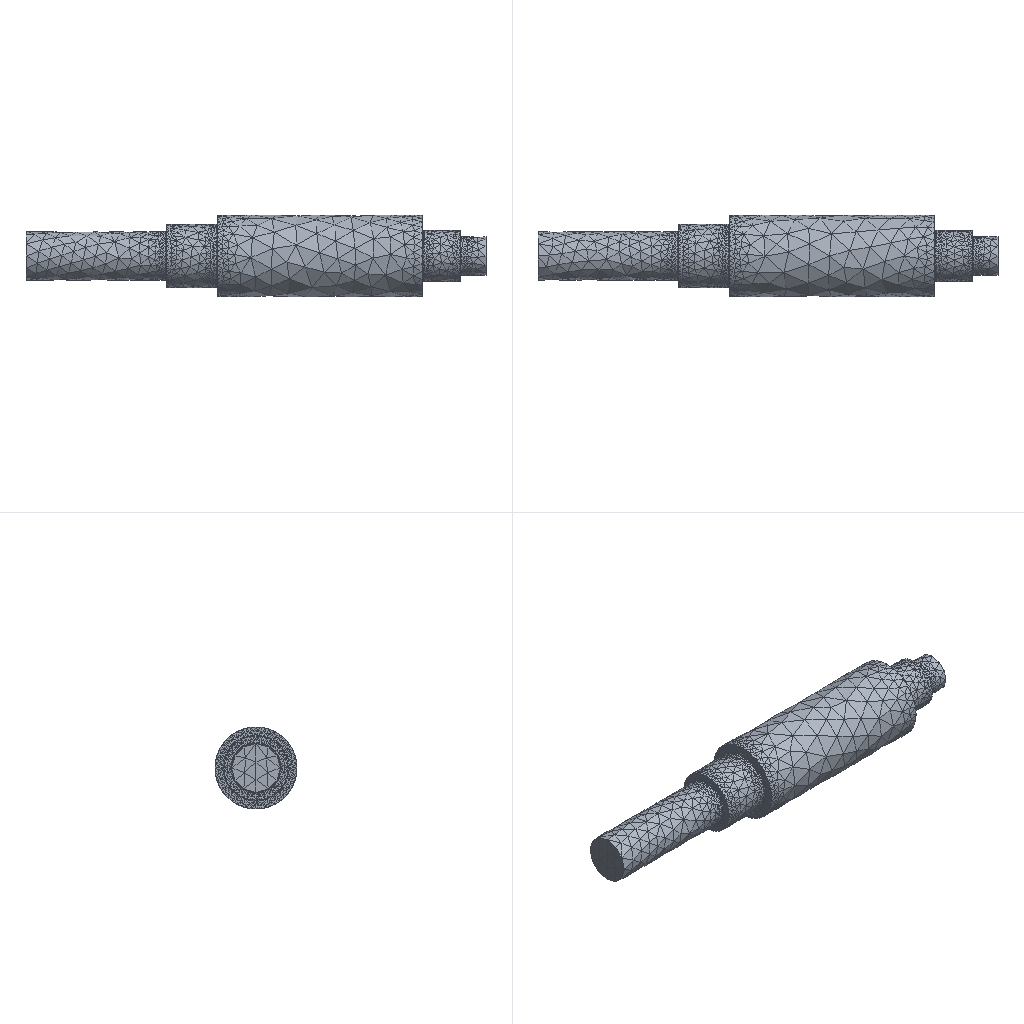Simulation study | ansys workbench
Set-up summary:
category,name,step,type,value,unit,region
solver,ansys_workbench
units,mm-N-s-tonne (MPa),,stated,"/units,MPA"
analysis,LS1,,modal,method=lanb; n_modes=20
load_step,LS1,LS1,modal
mesh,nodes,,,91403
mesh,elements,,,61675
element_type,SOLID187,,,61675
material,Structural Steel,,E,200000,tonne s^-2 mm^-1
material,Structural Steel,,nu,0.3
material,Structural Steel,,density,7.85e-09,tonne mm^-3
material,Structural Steel,,conductivity,60.5,tonne mm s^-3 C^-1
material,Structural Steel,,specific_heat,4.34e+08,mm^2 s^-2 C^-1
material,Structural Steel,,cte,1.2e-05,C^-1
material,Structural Steel,,permeability,10000
material,Structural Steel,,resistivity,0.00017,ohm mm
bc,Frictionless Supports X,model,fixed,[dofs=UX],,_FRICSUX
bc,Frictionless Supports Z,model,fixed,[dofs=UZ],,_FRICSUZ
named_set,_FRICSUX,,node,2114
named_set,_FRICSUZ,,node,2114
Ansys APDL input file, long lists of numbers shortened:
/batch
/config,noeldb,1     ! force off writing results to database
*get,_wallstrt,active,,time,wall
! ANSYS input file written by Workbench version 2025 R2
! File used for geometry attach:
/title,______________--__ (A5)
! ****** Begin Custom Load Command Snippet ******
/COM, ACT Extensions:
/COM,     LSDYNA, 2025.2
/COM,/COM,     ANSYSMotion, 2025.2
/COM,
! ****** End   Custom Load Command Snippet ******
*DIM,_wb_ProjectScratch_dir,string,248
_wb_ProjectScratch_dir(1) = ''
/com,--- Data in consistent NMM units. See Solving Units in the help system for more information.
/units,MPA
/nopr
/wb,file,start              !  signify a WB generated input file
/prep7
! Turn off shape checking because checks already performed inside WB mesher.
! See help system for more information.
SHPP,OFF,,NOWARN
/nolist
etcon,set             ! allow ANSYS to choose best KEYOP's for 180x elements, resets any applicable keyopt to MAPDL defaults
/com,*********** Send User Defined Coordinate System(s) ***********
csys,0
/com,*********** Nodes for the whole assembly ***********
nblock,3,,100543
(1i9,3e20.9e3)
        1     0.000000000E+00    -1.163414459E-15    -9.500000000E+00
! (91402 more lines like these left out)
-1
/wb,elem,start            !  set before creation of elements
/com,*********** Elements for Body 1 'Part 1' ***********
et,1,187
MAT,1 $ TYPE,1 $ REAL,1 $ SECNUM,1 $ ESYS,0
eblock,11,COMPACT,,61675
(11i9)
        1     7993    12675     8526     9142    67015    70402    67012    67013    74710    70396
! (61674 more lines like these left out)
-1
secnum,1    ! reset the section ID to default
/wb,elem,end               !  done creating elements
toffst,273.15,      ! Temperature offset from absolute zero
/com,*********** Set Reference Temperature ***********
tref,22.
/wb,mat,start              !  starting to send materials
/com,*********** Send Materials ***********
Temperature = 'TEMP' ! Temperature
MP,DENS,1,7.85e-09,	! tonne mm^-3
MP,ALPX,1,1.2e-05,	! C^-1
MP,C,1,434000000,	! mm^2 s^-2 C^-1
MP,KXX,1,60.5,	! tonne mm s^-3 C^-1
MP,RSVX,1,0.00017,	! ohm mm
MP,EX,1,200000,	! tonne s^-2 mm^-1
MP,NUXY,1,0.3,
MP,MURX,1,10000,
/wb,mat,end                !  done sending materials
!************************* Model Summary ********************
!Part 1,	结构钢,	matid,	1
!************************* End Model Summary ********************
! get the diagonal of the bounding box. Needed later for other things
*get,_xmin,node,,mnloc,x
*get,_ymin,node,,mnloc,y
*get,_zmin,node,,mnloc,z
*get,_xmax,node,,mxloc,x
*get,_ymax,node,,mxloc,y
*get,_zmax,node,,mxloc,z
_ASMDIAG=(_xmax-_xmin)*(_xmax-_xmin)+(_ymax-_ymin)*(_ymax-_ymin)+(_zmax-_zmin)*(_zmax-_zmin)
_ASMDIAG=SQRT(_ASMDIAG)
/wb,contact,start          !  starting to send contact
/wb,contact,end            !  done creating contacts
/golist
/wb,load,start             !  starting to send loads
/com,********* Frictionless Supports X *********
CMBLOCK,_FRICSUX,NODE,     2114
(8i10)
       262      -473      1125     -1234      1753     -1981      2597     -3039
! (264 more lines like these left out)
cmsel,s,_FRICSUX
d,all,ux,0
nsel,all
/com,********* Frictionless Supports Z *********
CMBLOCK,_FRICSUZ,NODE,     2114
(8i10)
       262      -473      1125     -1234      1753     -1981      2597     -3039
! (264 more lines like these left out)
cmsel,s,_FRICSUZ
d,all,uz,0
nsel,all
/com,*********** Node Rotations ***********
nmod,262,,,,-180.,0.,90.
nmod,263,,,,-180.,7.66,90.
nmod,264,,,,-180.,15.319,90.
nmod,265,,,,-180.,22.979,90.
! (3650 more lines like these left out)
/gst,on,on
fini
*get,_numnode,node,0,count
*get,_numelem,elem,0,count
*get, _MAXELEMNUM, elem, 0, NUM, MAX
*get, _MAXNODENUM, node, 0, NUM, MAX
*get, _MAXELEMTYPE, etyp, 0, NUM, MAX
*get, _MAXREALCONST, rcon, 0, NUM, MAX
/go
/wb,load,end               !  done creating loads
/com,--- Number of total nodes = %_numnode%
/com,--- Number of contact elements = 0
/com,--- Number of spring elements = 0
/com,--- Number of bearing elements = 0
/com,--- Number of solid elements = 61675
/com,--- Number of condensed parts = 0
/com,--- Number of total elements = %_numelem%
*get,_wallbsol,active,,time,wall
/solu
antype,2                   ! modal analysis
_thickRatio=  1     ! Ratio of thick parts in the model
thexpand,off     ! ignore thermal strains
modopt,lanb,20
outres,erase
outres,all,none
outres,nsol,all
outres,strs,all,
outres,epel,all,
outres,eppl,all,
mxpand,,,,yes,,no             ! expand requested element results, but not write them to file.mode
dmpopt,esav,no
dmpopt,emat,no
dmpopt,full,no
! *********** WB SOLVE COMMAND ***********
! check interactive state
*get,ANSINTER_,active,,int
*if,ANSINTER_,ne,0,then
/eof
*endif
solve
/com *************** Write FE CONNECTORS *********
CEWRITE,file,ce,,INTE
*get,_nmodalsolproc,active,0,numcpu
fini
/nopr
*get,_numnode,node,0,count
*get,_numelem,elem,0,count
*get, _MAXELEMNUM, elem, 0, NUM, MAX
*get, _MAXNODENUM, node, 0, NUM, MAX,,,INTERNAL
*get, _MAXELEMTYPE, etyp, 0, NUM, MAX
*get, _MAXREALCONST, rcon, 0, NUM, MAX
*get,_NSOLTHREADS,active,0,ntfs
*get,_NSOLPROCESSES,active,0,npfs
/gopr
*get,_wallasol,active,,time,wall
/post1
/nopr
*dim,_direction,CHAR,6,1
_direction(1) = 'X'
_direction(2) = 'Y'
_direction(3) = 'Z'
_direction(4) = 'ROTX'
_direction(5) = 'ROTY'
_direction(6) = 'ROTZ'
*get,_lastLS,active,0,set,LSTP
*get,_beginset,active,0,set,nset,first,_lastLS
*get,_endset,active,0,set,nset,last,_lastLS
_nummodes = 0
*if,_endset,gt,0,then
_nummodes = _endset - _beginset + 1
*endif
*do,i_mode,1,_nummodes
   *do,j_component,1,6
			*get,PFACT_%i_mode%_%j_component%,MODE,%i_mode%,PFACT,,DIREC,_direction(%j_component%)
   *enddo
*enddo
*dim,_tmdirection,CHAR,6,1
_tmdirection(1) = 'X'
_tmdirection(2) = 'Y'
_tmdirection(3) = 'Z'
_tmdirection(4) = 'X'
_tmdirection(5) = 'Y'
_tmdirection(6) = 'Z'
*do,j_component,1,6
    *if,j_component,gt,3,then
        *get,TOTALMASS_%j_component%,ELEM,0,IOR,_tmdirection(%j_component%)
    *else
        *get,TOTALMASS_%j_component%,ELEM,0,MTOT,_tmdirection(%j_component%)
    *endif
*enddo
/gopr
xmlo,ENCODING,ISO-8859-1
xmlo,parm
/xml,parm,xml
fini
/gopr
*get,_walldone,active,,time,wall
_preptime=(_wallbsol-_wallstrt)*3600
_solvtime=(_wallasol-_wallbsol)*3600
_posttime=(_walldone-_wallasol)*3600
_totaltim=(_walldone-_wallstrt)*3600
*get,_dlbratio,active,0,solu,dlbr
*get,_combtime,active,0,solu,comb
*get,_ssmode,active,0,solu,ssmm
*get,_ndofs,active,0,solu,ndof
/fclean				!clean distributed files
/com,--- Total number of nodes = %_numnode%
/com,--- Total number of elements = %_numelem%
/com,--- Element load balance ratio = %_dlbratio%
/com,--- Time to combine distributed files = %_combtime%
/com,--- Sparse memory mode = %_ssmode%
/com,--- Number of DOF = %_ndofs%
/wb,file,end               ! done with WB generated input
Results summary:
result,analyses[0].index,,,1
result,analyses[0].system,,,SYS
result,analyses[0].deck,,,deck.dat
result,analyses[0].solve_status,,,completed
result,analyses[0].analysis_type,,,modal
result,analyses[0].physics,,,mechanical
result,analyses[0].unit_system,,,"NMM: mm, ton, N, s, mV, mA, degC"
result,analyses[0].n_sets,,,20
result,analyses[0].modal_frequencies_hz[1],,,0
result,analyses[0].modal_frequencies_hz[2],,,3747.66
result,analyses[0].modal_frequencies_hz[3],,,3747.72
result,analyses[0].modal_frequencies_hz[4],,,7536.52
result,analyses[0].modal_frequencies_hz[5],,,7536.65
result,analyses[0].modal_frequencies_hz[6],,,11771.7
result,analyses[0].modal_frequencies_hz[7],,,17490
result,analyses[0].modal_frequencies_hz[8],,,17490.2
result,analyses[0].modal_frequencies_hz[9],,,18357.4
result,analyses[0].modal_frequencies_hz[10],,,18724.4
result,analyses[0].modal_frequencies_hz[11],,,18724.6
result,analyses[0].modal_frequencies_hz[12],,,19208.1
result,analyses[0].modal_frequencies_hz[13],,,20788.4
result,analyses[0].modal_frequencies_hz[14],,,30224.7
result,analyses[0].modal_frequencies_hz[15],,,31021
result,analyses[0].modal_frequencies_hz[16],,,31021.6
result,analyses[0].modal_frequencies_hz[17],,,36283.7
result,analyses[0].modal_frequencies_hz[18],,,42178.1
result,analyses[0].modal_frequencies_hz[19],,,42179.1
result,analyses[0].modal_frequencies_hz[20],,,42236.6